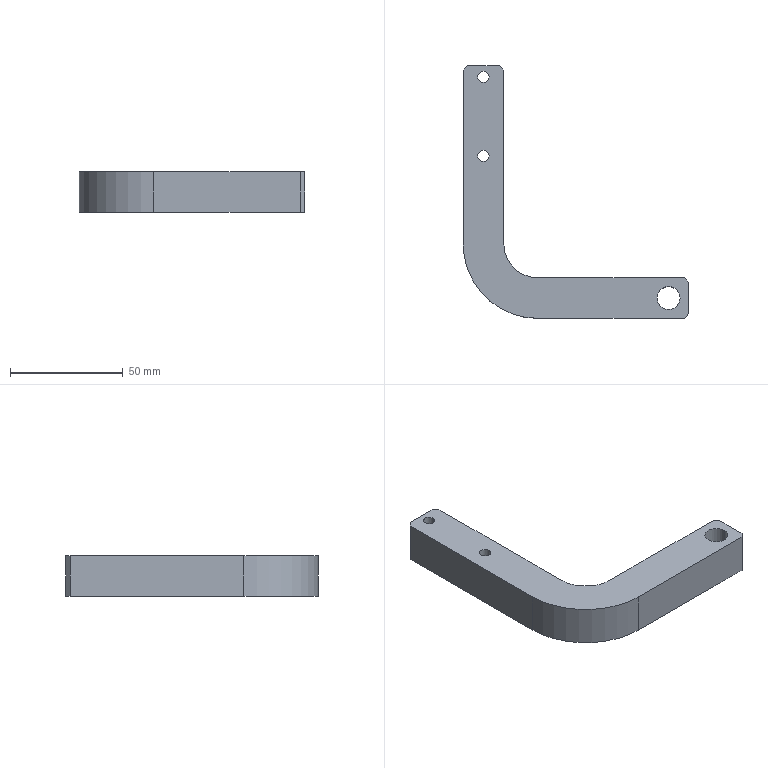Part | STEP file | YCD14007A-08.03.07.06 Limit Rod | 1 solid | 20 faces | box 100 x 112 x 18 mm | volume 57197 mm3 | plane 12 | cylinder 8 | commonest cylinder face diameters 5 x4 10.2 x2 30 x1 66 x1